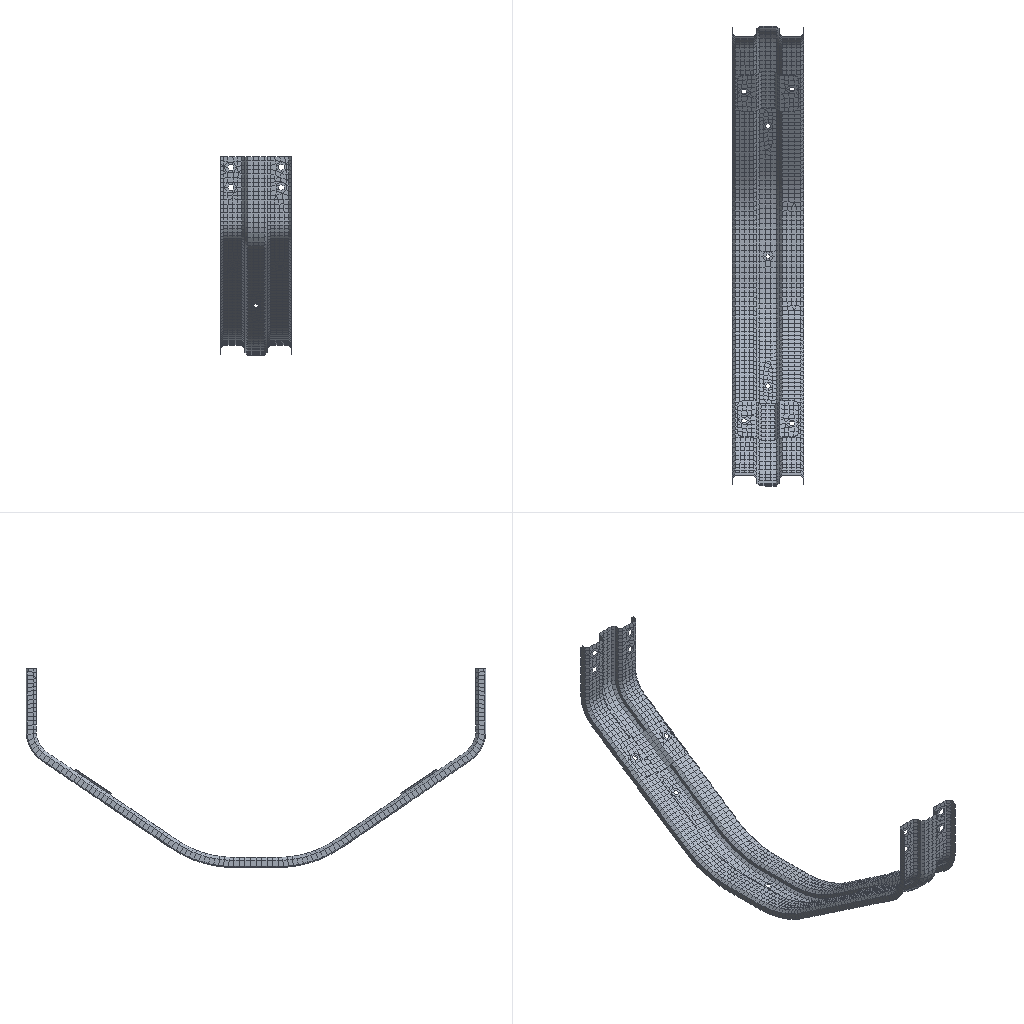Simulation study | nastran
Set-up summary:
category,name,step,type,value,unit,region
solver,nx_nastran
units,not stated in the deck,,not stated
analysis,deck,,modal,modal
analysis,solution,,SOL,103
load_step,SUBCASE 1,1,SUBCASE,SPC=1 LOAD=None
mesh,nodes,,,3434
mesh,elements,,,3210
element_type,CQUAD4,,shell,3136
element_type,CTRIA3,,shell,74
load,load commands in deck,,count,0
bc,support commands in deck,,count,8
check,setup vs results,,match,"every grid point's frame and coordinates and every element id; grid points of CQUAD4, CTRIA3 elements"
Nastran input file, long lists of numbers shortened:
$$------------------------------------------------------------------------------$
$$                                                                              $
$$ NASTRAN Input Deck Generated by HyperMesh Version  :10.0buil                 $
$$ Generated using HyperMesh-Nastran Template Version : 10.0build60
$$                                                                              $
$$   Template:  general                                                         $
$$                                                                              $
$$------------------------------------------------------------------------------$
$$------------------------------------------------------------------------------$
$$                      Executive Control Cards                                 $
$$------------------------------------------------------------------------------$
SOL 103
CEND
$$------------------------------------------------------------------------------$
$$                      Case Control Cards                                      $
$$------------------------------------------------------------------------------$
  DISPLACEMENT = ALL
$
$HMNAME LOADSTEP               1"3"
SUBCASE       1
  LABEL= 3
  SPC =        1
  METHOD(STRUCTURE) =        2
$$------------------------------------------------------------------------------$
$$                      Bulk Data Cards                                         $
$$------------------------------------------------------------------------------$
BEGIN BULK
PARAM,POST,-1
$$
$$  GRID Data
$$
GRID        7022        1172.0  -358.774-325.977
GRID        7751        1153.0  -331.161-344.601
$ (3432 more lines like these left out)
$$
$$  SPOINT Data
$$
$$
$$------------------------------------------------------------------------------$
$$             Group Definitions                                                $
$$------------------------------------------------------------------------------$
$$
$$ RBE2 Elements - Multiple dependent nodes
$$
RBE2      202722  238068  123456   43148   43150   43164   43166   43167+
+          43171  231786  231787  231788  231789  231790  231791  231825+
+         231833  231834  231839  231843  231844  232299  232300  232301+
+         232302  232303  232304
RBE2      202723  238069  123456   43092   43093   43094   43097   43100+
+          43127  231679  231680  231681  231682  231683  231684  231826+
+         231827  231828  231830  231840  231842  232294  232295  232296+
+         232297  232298  232836
$ (24 more lines like these left out)
$
$HMMOVE 10010022
$         202722THRU      202725  202728  202730THRU      202736
$
$$
$$  CTRIA3 Data
$$
CTRIA3     40309       2   41652   41656   41637
CTRIA3     40711       2   42056   42065   42055
$ (72 more lines like these left out)
$
$HMMOVE 10010016
$          40309   40711   40772   40774   40777   41220   41228   41240   41249
$          41251   41255   41257   41259   41261   41265   41269   41273   41279
$          41283   41288THRU       41289   41333   41341   41348   41356THRU
$          41357   41550   41888   41906   41911   41915  198533   42598   42602
$          42613   42623   42628   42681   42687   42689   42691   42693   42696
$         198823  198840  198842  198969  198980  198989  198992THRU      198993
$         198997THRU      198998  202691
$
$
$HMMOVE 10010018
$          41373   41377   41384   41391   41396   41398   41488   41492   41495
$       THRU       41496   43225THRU       43227   43236  199086  199088  199093
$         199100  199107  199111
$
$
$  CQUAD4 Elements
$
CQUAD4    197193       2  237093  237094  237106  237092
CQUAD4    197194       2  237105  237107  237110  237109
$ (3134 more lines like these left out)
$
$HMMOVE 10010016
$         197193THRU      197195  197995THRU      197999  198001THRU      198009
$         198014  198052THRU      198054  198057THRU      198058  198060THRU
$ (98 more lines like these left out)
PSHELL         1       13.5            1               1
$
$HMNAME PROP                   2"400t" 4
$HWCOLOR PROP                  2      11
PSHELL         2       14.0            1               1
$$
$$------------------------------------------------------------------------------$
$$                      Material Definition Cards                               $
$$------------------------------------------------------------------------------$
$$--------------------------------------------------------------
$$ HYPERMESH TAGS
$$--------------------------------------------------------------
$$BEGIN TAGS
$$END TAGS
$$
$$  MAT1 Data
$
$HMNAME MAT                    1"steel" "MAT1"
$HWCOLOR MAT                   1      11
MAT1           1210000.0        0.3     7.85E-09
$$
$$
$$
$$------------------------------------------------------------------------------$
$ (34 more lines like these left out)
EIGRL          20.0                    5                            MASS
$$
$$  SPC Data
$$
SPC            1  238078  1234560.0
SPC            1  238077  1234560.0
SPC            1  238076  1234560.0
SPC            1  238074  1234560.0
SPC            1  238081  1234560.0
SPC            1  238082  1234560.0
SPC            1  238080  1234560.0
SPC            1  238079  1234560.0
$HMASSEM   10010       5 1001
$HMASSEM_IDS    1001001610010018
$
ENDDATA
Results summary:
result,analysis,,,modal
result,primary field,,,eigenvectors